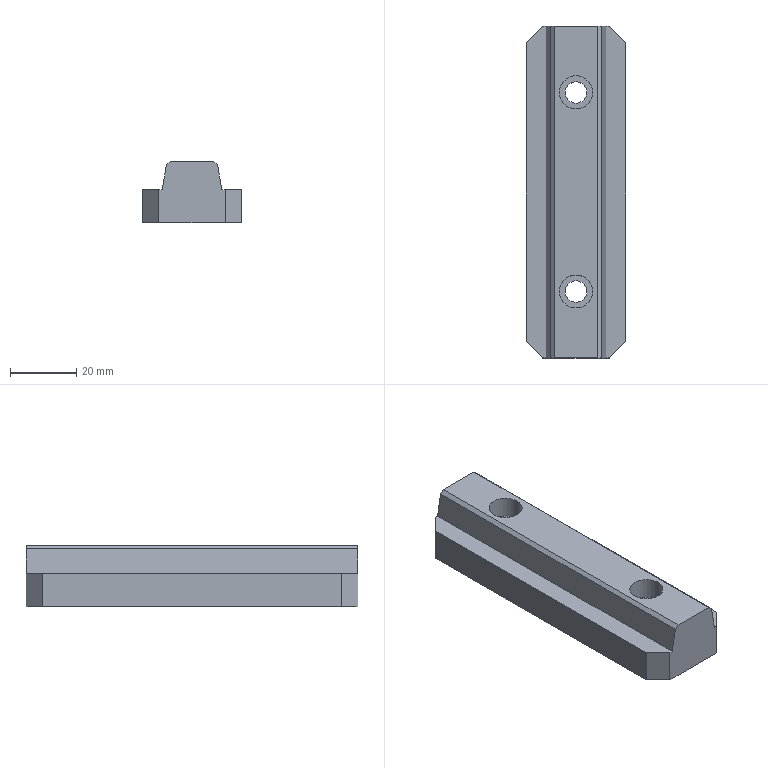Part | Creo | 1 solid | 26 faces | box 30 x 100 x 18.5 mm | volume 41610 mm3 | plane 18 | cylinder 8 | commonest cylinder face diameters 6.5 x4 10 x4
STEP:
#1=CARTESIAN_POINT('',(-253.501,30.,8.5));
#2=VERTEX_POINT('',#1);
#3=CARTESIAN_POINT('',(-240.499,30.,8.5));
#4=VERTEX_POINT('',#3);
#5=CARTESIAN_POINT('',(-253.501,30.,8.5));
#6=DIRECTION('',(1.,0.,0.));
#7=VECTOR('',#6,13.002);
#8=LINE('',#5,#7);
#9=EDGE_CURVE('',#2,#4,#8,.T.);
#10=ORIENTED_EDGE('',*,*,#9,.F.);
#11=CARTESIAN_POINT('',(-253.501,130.,8.5));
#12=VERTEX_POINT('',#11);
#13=CARTESIAN_POINT('',(-253.501,30.,8.5));
#14=DIRECTION('',(0.,1.,0.));
#15=VECTOR('',#14,100.);
#16=LINE('',#13,#15);
#17=EDGE_CURVE('',#2,#12,#16,.T.);
#18=ORIENTED_EDGE('',*,*,#17,.T.);
#19=CARTESIAN_POINT('',(-240.499,130.,8.5));
#20=VERTEX_POINT('',#19);
#21=CARTESIAN_POINT('',(-253.501,130.,8.5));
#22=DIRECTION('',(1.,0.,0.));
#23=VECTOR('',#22,13.002);
#24=LINE('',#21,#23);
#25=EDGE_CURVE('',#12,#20,#24,.T.);
#26=ORIENTED_EDGE('',*,*,#25,.T.);
#27=CARTESIAN_POINT('',(-240.499,130.,8.5));
#28=DIRECTION('',(0.,-1.,0.));
#29=VECTOR('',#28,100.);
#30=LINE('',#27,#29);
#31=EDGE_CURVE('',#20,#4,#30,.T.);
#32=ORIENTED_EDGE('',*,*,#31,.T.);
#33=EDGE_LOOP('',(#10,#18,#26,#32));
#34=FACE_OUTER_BOUND('',#33,.F.);
#35=CARTESIAN_POINT('',(-252.,50.,8.5));
#36=VERTEX_POINT('',#35);
#37=CARTESIAN_POINT('',(-242.,50.,8.5));
#38=VERTEX_POINT('',#37);
#39=CARTESIAN_POINT('',(-247.,50.,8.5));
#40=DIRECTION('',(0.,0.,-1.));
#41=DIRECTION('',(-1.,0.,0.));
#42=AXIS2_PLACEMENT_3D('',#39,#40,#41);
#43=CIRCLE('',#42,5.);
#44=EDGE_CURVE('',#36,#38,#43,.T.);
#45=ORIENTED_EDGE('',*,*,#44,.F.);
#46=CARTESIAN_POINT('',(-247.,50.,8.5));
#47=DIRECTION('',(0.,0.,-1.));
#48=DIRECTION('',(1.,0.,0.));
#49=AXIS2_PLACEMENT_3D('',#46,#47,#48);
#50=CIRCLE('',#49,5.);
#51=EDGE_CURVE('',#38,#36,#50,.T.);
#52=ORIENTED_EDGE('',*,*,#51,.F.);
#53=EDGE_LOOP('',(#45,#52));
#54=FACE_BOUND('',#53,.F.);
#55=CARTESIAN_POINT('',(-252.,110.,8.5));
#56=VERTEX_POINT('',#55);
#57=CARTESIAN_POINT('',(-242.,110.,8.5));
#58=VERTEX_POINT('',#57);
#59=CARTESIAN_POINT('',(-247.,110.,8.5));
#60=DIRECTION('',(0.,0.,-1.));
#61=DIRECTION('',(-1.,0.,0.));
#62=AXIS2_PLACEMENT_3D('',#59,#60,#61);
#63=CIRCLE('',#62,5.);
#64=EDGE_CURVE('',#56,#58,#63,.T.);
#65=ORIENTED_EDGE('',*,*,#64,.F.);
#66=CARTESIAN_POINT('',(-247.,110.,8.5));
#67=DIRECTION('',(0.,0.,-1.));
#68=DIRECTION('',(1.,0.,0.));
#69=AXIS2_PLACEMENT_3D('',#66,#67,#68);
#70=CIRCLE('',#69,5.);
#71=EDGE_CURVE('',#58,#56,#70,.T.);
#72=ORIENTED_EDGE('',*,*,#71,.F.);
#73=EDGE_LOOP('',(#65,#72));
#74=FACE_BOUND('',#73,.F.);
#75=CARTESIAN_POINT('',(-239.499,130.,8.5));
#76=DIRECTION('',(0.,0.,1.));
#77=DIRECTION('',(1.,0.,0.));
#78=AXIS2_PLACEMENT_3D('',#75,#76,#77);
#79=PLANE('',#78);
#80=ADVANCED_FACE('',(#34,#54,#74),#79,.T.);
#81=CARTESIAN_POINT('',(-242.,50.,2.));
#82=VERTEX_POINT('',#81);
#83=CARTESIAN_POINT('',(-252.,50.,2.));
#84=VERTEX_POINT('',#83);
#85=CARTESIAN_POINT('',(-247.,50.,2.));
#86=DIRECTION('',(0.,0.,1.));
#87=DIRECTION('',(1.,0.,0.));
#88=AXIS2_PLACEMENT_3D('',#85,#86,#87);
#89=CIRCLE('',#88,5.);
#90=EDGE_CURVE('',#82,#84,#89,.T.);
#91=ORIENTED_EDGE('',*,*,#90,.T.);
#92=CARTESIAN_POINT('',(-252.,50.,8.5));
#93=DIRECTION('',(0.,0.,-1.));
#94=VECTOR('',#93,6.5);
#95=LINE('',#92,#94);
#96=EDGE_CURVE('',#36,#84,#95,.T.);
#97=ORIENTED_EDGE('',*,*,#96,.F.);
#98=ORIENTED_EDGE('',*,*,#44,.T.);
#99=CARTESIAN_POINT('',(-242.,50.,8.5));
#100=DIRECTION('',(0.,0.,-1.));
#101=VECTOR('',#100,6.5);
#102=LINE('',#99,#101);
#103=EDGE_CURVE('',#38,#82,#102,.T.);
#104=ORIENTED_EDGE('',*,*,#103,.T.);
#105=EDGE_LOOP('',(#91,#97,#98,#104));
#106=FACE_OUTER_BOUND('',#105,.F.);
#107=CARTESIAN_POINT('',(-247.,50.,8.5));
#108=DIRECTION('',(0.,0.,-1.));
#109=DIRECTION('',(-1.,0.,0.));
#110=AXIS2_PLACEMENT_3D('',#107,#108,#109);
#111=CYLINDRICAL_SURFACE('',#110,5.);
#112=ADVANCED_FACE('',(#106),#111,.F.);
#113=ORIENTED_EDGE('',*,*,#90,.F.);
#114=CARTESIAN_POINT('',(-247.,50.,2.));
#115=DIRECTION('',(0.,0.,1.));
#116=DIRECTION('',(-1.,0.,0.));
#117=AXIS2_PLACEMENT_3D('',#114,#115,#116);
#118=CIRCLE('',#117,5.);
#119=EDGE_CURVE('',#84,#82,#118,.T.);
#120=ORIENTED_EDGE('',*,*,#119,.F.);
#121=EDGE_LOOP('',(#113,#120));
#122=FACE_OUTER_BOUND('',#121,.F.);
#123=CARTESIAN_POINT('',(-250.25,50.,2.));
#124=VERTEX_POINT('',#123);
#125=CARTESIAN_POINT('',(-243.75,50.,2.));
#126=VERTEX_POINT('',#125);
#127=CARTESIAN_POINT('',(-247.,50.,2.));
#128=DIRECTION('',(0.,0.,-1.));
#129=DIRECTION('',(-1.,0.,0.));
#130=AXIS2_PLACEMENT_3D('',#127,#128,#129);
#131=CIRCLE('',#130,3.25);
#132=EDGE_CURVE('',#124,#126,#131,.T.);
#133=ORIENTED_EDGE('',*,*,#132,.F.);
#134=CARTESIAN_POINT('',(-247.,50.,2.));
#135=DIRECTION('',(0.,0.,-1.));
#136=DIRECTION('',(1.,0.,0.));
#137=AXIS2_PLACEMENT_3D('',#134,#135,#136);
#138=CIRCLE('',#137,3.25);
#139=EDGE_CURVE('',#126,#124,#138,.T.);
#140=ORIENTED_EDGE('',*,*,#139,.F.);
#141=EDGE_LOOP('',(#133,#140));
#142=FACE_BOUND('',#141,.F.);
#143=CARTESIAN_POINT('',(-247.,50.,2.));
#144=DIRECTION('',(0.,0.,-1.));
#145=DIRECTION('',(-1.,0.,0.));
#146=AXIS2_PLACEMENT_3D('',#143,#144,#145);
#147=PLANE('',#146);
#148=ADVANCED_FACE('',(#122,#142),#147,.F.);
#149=ORIENTED_EDGE('',*,*,#119,.T.);
#150=ORIENTED_EDGE('',*,*,#103,.F.);
#151=ORIENTED_EDGE('',*,*,#51,.T.);
#152=ORIENTED_EDGE('',*,*,#96,.T.);
#153=EDGE_LOOP('',(#149,#150,#151,#152));
#154=FACE_OUTER_BOUND('',#153,.F.);
#155=CARTESIAN_POINT('',(-247.,50.,8.5));
#156=DIRECTION('',(0.,0.,-1.));
#157=DIRECTION('',(-1.,0.,0.));
#158=AXIS2_PLACEMENT_3D('',#155,#156,#157);
#159=CYLINDRICAL_SURFACE('',#158,5.);
#160=ADVANCED_FACE('',(#154),#159,.F.);
#161=ORIENTED_EDGE('',*,*,#132,.T.);
#162=CARTESIAN_POINT('',(-243.75,50.,-10.));
#163=VERTEX_POINT('',#162);
#164=CARTESIAN_POINT('',(-243.75,50.,2.));
#165=DIRECTION('',(0.,0.,-1.));
#166=VECTOR('',#165,12.);
#167=LINE('',#164,#166);
#168=EDGE_CURVE('',#126,#163,#167,.T.);
#169=ORIENTED_EDGE('',*,*,#168,.T.);
#170=CARTESIAN_POINT('',(-250.25,50.,-10.));
#171=VERTEX_POINT('',#170);
#172=CARTESIAN_POINT('',(-247.,50.,-10.));
#173=DIRECTION('',(0.,0.,1.));
#174=DIRECTION('',(1.,0.,0.));
#175=AXIS2_PLACEMENT_3D('',#172,#173,#174);
#176=CIRCLE('',#175,3.25);
#177=EDGE_CURVE('',#163,#171,#176,.T.);
#178=ORIENTED_EDGE('',*,*,#177,.T.);
#179=CARTESIAN_POINT('',(-250.25,50.,2.));
#180=DIRECTION('',(0.,0.,-1.));
#181=VECTOR('',#180,12.);
#182=LINE('',#179,#181);
#183=EDGE_CURVE('',#124,#171,#182,.T.);
#184=ORIENTED_EDGE('',*,*,#183,.F.);
#185=EDGE_LOOP('',(#161,#169,#178,#184));
#186=FACE_OUTER_BOUND('',#185,.F.);
#187=CARTESIAN_POINT('',(-247.,50.,8.5));
#188=DIRECTION('',(0.,0.,-1.));
#189=DIRECTION('',(-1.,0.,0.));
#190=AXIS2_PLACEMENT_3D('',#187,#188,#189);
#191=CYLINDRICAL_SURFACE('',#190,3.25);
#192=ADVANCED_FACE('',(#186),#191,.F.);
#193=ORIENTED_EDGE('',*,*,#139,.T.);
#194=ORIENTED_EDGE('',*,*,#183,.T.);
#195=CARTESIAN_POINT('',(-247.,50.,-10.));
#196=DIRECTION('',(0.,0.,1.));
#197=DIRECTION('',(-1.,0.,0.));
#198=AXIS2_PLACEMENT_3D('',#195,#196,#197);
#199=CIRCLE('',#198,3.25);
#200=EDGE_CURVE('',#171,#163,#199,.T.);
#201=ORIENTED_EDGE('',*,*,#200,.T.);
#202=ORIENTED_EDGE('',*,*,#168,.F.);
#203=EDGE_LOOP('',(#193,#194,#201,#202));
#204=FACE_OUTER_BOUND('',#203,.F.);
#205=CARTESIAN_POINT('',(-247.,50.,8.5));
#206=DIRECTION('',(0.,0.,-1.));
#207=DIRECTION('',(-1.,0.,0.));
#208=AXIS2_PLACEMENT_3D('',#205,#206,#207);
#209=CYLINDRICAL_SURFACE('',#208,3.25);
#210=ADVANCED_FACE('',(#204),#209,.F.);
#211=CARTESIAN_POINT('',(-262.,35.,-10.));
#212=VERTEX_POINT('',#211);
#213=CARTESIAN_POINT('',(-262.,125.,-10.));
#214=VERTEX_POINT('',#213);
#215=CARTESIAN_POINT('',(-262.,35.,-10.));
#216=DIRECTION('',(0.,1.,0.));
#217=VECTOR('',#216,90.);
#218=LINE('',#215,#217);
#219=EDGE_CURVE('',#212,#214,#218,.T.);
#220=ORIENTED_EDGE('',*,*,#219,.F.);
#221=CARTESIAN_POINT('',(-257.,30.,-10.));
#222=VERTEX_POINT('',#221);
#223=CARTESIAN_POINT('',(-257.,30.,-10.));
#224=DIRECTION('',(-0.7071,0.7071,0.));
#225=VECTOR('',#224,7.071);
#226=LINE('',#223,#225);
#227=EDGE_CURVE('',#222,#212,#226,.T.);
#228=ORIENTED_EDGE('',*,*,#227,.F.);
#229=CARTESIAN_POINT('',(-237.,30.,-10.));
#230=VERTEX_POINT('',#229);
#231=CARTESIAN_POINT('',(-237.,30.,-10.));
#232=DIRECTION('',(-1.,0.,0.));
#233=VECTOR('',#232,20.);
#234=LINE('',#231,#233);
#235=EDGE_CURVE('',#230,#222,#234,.T.);
#236=ORIENTED_EDGE('',*,*,#235,.F.);
#237=CARTESIAN_POINT('',(-232.,35.,-10.));
#238=VERTEX_POINT('',#237);
#239=CARTESIAN_POINT('',(-232.,35.,-10.));
#240=DIRECTION('',(-0.7071,-0.7071,0.));
#241=VECTOR('',#240,7.071);
#242=LINE('',#239,#241);
#243=EDGE_CURVE('',#238,#230,#242,.T.);
#244=ORIENTED_EDGE('',*,*,#243,.F.);
#245=CARTESIAN_POINT('',(-232.,125.,-10.));
#246=VERTEX_POINT('',#245);
#247=CARTESIAN_POINT('',(-232.,125.,-10.));
#248=DIRECTION('',(0.,-1.,0.));
#249=VECTOR('',#248,90.);
#250=LINE('',#247,#249);
#251=EDGE_CURVE('',#246,#238,#250,.T.);
#252=ORIENTED_EDGE('',*,*,#251,.F.);
#253=CARTESIAN_POINT('',(-237.,130.,-10.));
#254=VERTEX_POINT('',#253);
#255=CARTESIAN_POINT('',(-237.,130.,-10.));
#256=DIRECTION('',(0.7071,-0.7071,0.));
#257=VECTOR('',#256,7.071);
#258=LINE('',#255,#257);
#259=EDGE_CURVE('',#254,#246,#258,.T.);
#260=ORIENTED_EDGE('',*,*,#259,.F.);
#261=CARTESIAN_POINT('',(-257.,130.,-10.));
#262=VERTEX_POINT('',#261);
#263=CARTESIAN_POINT('',(-257.,130.,-10.));
#264=DIRECTION('',(1.,0.,0.));
#265=VECTOR('',#264,20.);
#266=LINE('',#263,#265);
#267=EDGE_CURVE('',#262,#254,#266,.T.);
#268=ORIENTED_EDGE('',*,*,#267,.F.);
#269=CARTESIAN_POINT('',(-262.,125.,-10.));
#270=DIRECTION('',(0.7071,0.7071,0.));
#271=VECTOR('',#270,7.071);
#272=LINE('',#269,#271);
#273=EDGE_CURVE('',#214,#262,#272,.T.);
#274=ORIENTED_EDGE('',*,*,#273,.F.);
#275=EDGE_LOOP('',(#220,#228,#236,#244,#252,#260,#268,#274));
#276=FACE_OUTER_BOUND('',#275,.F.);
#277=CARTESIAN_POINT('',(-243.75,110.,-10.));
#278=VERTEX_POINT('',#277);
#279=CARTESIAN_POINT('',(-250.25,110.,-10.));
#280=VERTEX_POINT('',#279);
#281=CARTESIAN_POINT('',(-247.,110.,-10.));
#282=DIRECTION('',(0.,0.,1.));
#283=DIRECTION('',(1.,0.,0.));
#284=AXIS2_PLACEMENT_3D('',#281,#282,#283);
#285=CIRCLE('',#284,3.25);
#286=EDGE_CURVE('',#278,#280,#285,.T.);
#287=ORIENTED_EDGE('',*,*,#286,.F.);
#288=CARTESIAN_POINT('',(-247.,110.,-10.));
#289=DIRECTION('',(0.,0.,1.));
#290=DIRECTION('',(-1.,0.,0.));
#291=AXIS2_PLACEMENT_3D('',#288,#289,#290);
#292=CIRCLE('',#291,3.25);
#293=EDGE_CURVE('',#280,#278,#292,.T.);
#294=ORIENTED_EDGE('',*,*,#293,.F.);
#295=EDGE_LOOP('',(#287,#294));
#296=FACE_BOUND('',#295,.F.);
#297=ORIENTED_EDGE('',*,*,#177,.F.);
#298=ORIENTED_EDGE('',*,*,#200,.F.);
#299=EDGE_LOOP('',(#297,#298));
#300=FACE_BOUND('',#299,.F.);
#301=CARTESIAN_POINT('',(-247.,80.,-10.));
#302=DIRECTION('',(0.,0.,-1.));
#303=DIRECTION('',(-1.,0.,0.));
#304=AXIS2_PLACEMENT_3D('',#301,#302,#303);
#305=PLANE('',#304);
#306=ADVANCED_FACE('',(#276,#296,#300),#305,.T.);
#307=CARTESIAN_POINT('',(-262.,125.,0.));
#308=VERTEX_POINT('',#307);
#309=CARTESIAN_POINT('',(-262.,35.,0.));
#310=VERTEX_POINT('',#309);
#311=CARTESIAN_POINT('',(-262.,125.,0.));
#312=DIRECTION('',(0.,-1.,0.));
#313=VECTOR('',#312,90.);
#314=LINE('',#311,#313);
#315=EDGE_CURVE('',#308,#310,#314,.T.);
#316=ORIENTED_EDGE('',*,*,#315,.T.);
#317=CARTESIAN_POINT('',(-262.,35.,0.));
#318=DIRECTION('',(0.,0.,-1.));
#319=VECTOR('',#318,10.);
#320=LINE('',#317,#319);
#321=EDGE_CURVE('',#310,#212,#320,.T.);
#322=ORIENTED_EDGE('',*,*,#321,.T.);
#323=ORIENTED_EDGE('',*,*,#219,.T.);
#324=CARTESIAN_POINT('',(-262.,125.,-10.));
#325=DIRECTION('',(0.,0.,1.));
#326=VECTOR('',#325,10.);
#327=LINE('',#324,#326);
#328=EDGE_CURVE('',#214,#308,#327,.T.);
#329=ORIENTED_EDGE('',*,*,#328,.T.);
#330=EDGE_LOOP('',(#316,#322,#323,#329));
#331=FACE_OUTER_BOUND('',#330,.F.);
#332=CARTESIAN_POINT('',(-262.,80.,-10.));
#333=DIRECTION('',(-1.,0.,0.));
#334=DIRECTION('',(0.,0.,1.));
#335=AXIS2_PLACEMENT_3D('',#332,#333,#334);
#336=PLANE('',#335);
#337=ADVANCED_FACE('',(#331),#336,.T.);
#338=CARTESIAN_POINT('',(-256.,30.,0.));
#339=VERTEX_POINT('',#338);
#340=CARTESIAN_POINT('',(-256.,130.,0.));
#341=VERTEX_POINT('',#340);
#342=CARTESIAN_POINT('',(-256.,30.,0.));
#343=DIRECTION('',(0.,1.,0.));
#344=VECTOR('',#343,100.);
#345=LINE('',#342,#344);
#346=EDGE_CURVE('',#339,#341,#345,.T.);
#347=ORIENTED_EDGE('',*,*,#346,.F.);
#348=CARTESIAN_POINT('',(-257.,30.,0.));
#349=VERTEX_POINT('',#348);
#350=CARTESIAN_POINT('',(-257.,30.,0.));
#351=DIRECTION('',(1.,0.,0.));
#352=VECTOR('',#351,1.);
#353=LINE('',#350,#352);
#354=EDGE_CURVE('',#349,#339,#353,.T.);
#355=ORIENTED_EDGE('',*,*,#354,.F.);
#356=CARTESIAN_POINT('',(-262.,35.,0.));
#357=DIRECTION('',(0.7071,-0.7071,0.));
#358=VECTOR('',#357,7.071);
#359=LINE('',#356,#358);
#360=EDGE_CURVE('',#310,#349,#359,.T.);
#361=ORIENTED_EDGE('',*,*,#360,.F.);
#362=ORIENTED_EDGE('',*,*,#315,.F.);
#363=CARTESIAN_POINT('',(-257.,130.,0.));
#364=VERTEX_POINT('',#363);
#365=CARTESIAN_POINT('',(-257.,130.,0.));
#366=DIRECTION('',(-0.7071,-0.7071,0.));
#367=VECTOR('',#366,7.071);
#368=LINE('',#365,#367);
#369=EDGE_CURVE('',#364,#308,#368,.T.);
#370=ORIENTED_EDGE('',*,*,#369,.F.);
#371=CARTESIAN_POINT('',(-256.,130.,0.));
#372=DIRECTION('',(-1.,0.,0.));
#373=VECTOR('',#372,1.);
#374=LINE('',#371,#373);
#375=EDGE_CURVE('',#341,#364,#374,.T.);
#376=ORIENTED_EDGE('',*,*,#375,.F.);
#377=EDGE_LOOP('',(#347,#355,#361,#362,#370,#376));
#378=FACE_OUTER_BOUND('',#377,.F.);
#379=CARTESIAN_POINT('',(-247.,80.,0.));
#380=DIRECTION('',(0.,0.,1.));
#381=DIRECTION('',(1.,0.,0.));
#382=AXIS2_PLACEMENT_3D('',#379,#380,#381);
#383=PLANE('',#382);
#384=ADVANCED_FACE('',(#378),#383,.T.);
#385=CARTESIAN_POINT('',(-254.675,30.,7.515));
#386=VERTEX_POINT('',#385);
#387=CARTESIAN_POINT('',(-254.675,30.,7.515));
#388=DIRECTION('',(-0.1736,0.,-0.9848));
#389=VECTOR('',#388,7.631);
#390=LINE('',#387,#389);
#391=EDGE_CURVE('',#386,#339,#390,.T.);
#392=ORIENTED_EDGE('',*,*,#391,.T.);
#393=ORIENTED_EDGE('',*,*,#346,.T.);
#394=CARTESIAN_POINT('',(-254.675,130.,7.515));
#395=VERTEX_POINT('',#394);
#396=CARTESIAN_POINT('',(-256.,130.,0.));
#397=DIRECTION('',(0.1736,0.,0.9848));
#398=VECTOR('',#397,7.631);
#399=LINE('',#396,#398);
#400=EDGE_CURVE('',#341,#395,#399,.T.);
#401=ORIENTED_EDGE('',*,*,#400,.T.);
#402=CARTESIAN_POINT('',(-254.675,130.,7.515));
#403=DIRECTION('',(0.,-1.,0.));
#404=VECTOR('',#403,100.);
#405=LINE('',#402,#404);
#406=EDGE_CURVE('',#395,#386,#405,.T.);
#407=ORIENTED_EDGE('',*,*,#406,.T.);
#408=EDGE_LOOP('',(#392,#393,#401,#407));
#409=FACE_OUTER_BOUND('',#408,.F.);
#410=CARTESIAN_POINT('',(-254.501,130.,8.5));
#411=DIRECTION('',(-0.9848,0.,0.1736));
#412=DIRECTION('',(0.1736,0.,0.9848));
#413=AXIS2_PLACEMENT_3D('',#410,#411,#412);
#414=PLANE('',#413);
#415=ADVANCED_FACE('',(#409),#414,.T.);
#416=CARTESIAN_POINT('',(-238.,30.,0.));
#417=VERTEX_POINT('',#416);
#418=CARTESIAN_POINT('',(-239.325,30.,7.515));
#419=VERTEX_POINT('',#418);
#420=CARTESIAN_POINT('',(-238.,30.,0.));
#421=DIRECTION('',(-0.1736,0.,0.9848));
#422=VECTOR('',#421,7.631);
#423=LINE('',#420,#422);
#424=EDGE_CURVE('',#417,#419,#423,.T.);
#425=ORIENTED_EDGE('',*,*,#424,.F.);
#426=CARTESIAN_POINT('',(-237.,30.,0.));
#427=VERTEX_POINT('',#426);
#428=CARTESIAN_POINT('',(-238.,30.,0.));
#429=DIRECTION('',(1.,0.,0.));
#430=VECTOR('',#429,1.);
#431=LINE('',#428,#430);
#432=EDGE_CURVE('',#417,#427,#431,.T.);
#433=ORIENTED_EDGE('',*,*,#432,.T.);
#434=CARTESIAN_POINT('',(-237.,30.,0.));
#435=DIRECTION('',(0.,0.,-1.));
#436=VECTOR('',#435,10.);
#437=LINE('',#434,#436);
#438=EDGE_CURVE('',#427,#230,#437,.T.);
#439=ORIENTED_EDGE('',*,*,#438,.T.);
#440=ORIENTED_EDGE('',*,*,#235,.T.);
#441=CARTESIAN_POINT('',(-257.,30.,-10.));
#442=DIRECTION('',(0.,0.,1.));
#443=VECTOR('',#442,10.);
#444=LINE('',#441,#443);
#445=EDGE_CURVE('',#222,#349,#444,.T.);
#446=ORIENTED_EDGE('',*,*,#445,.T.);
#447=ORIENTED_EDGE('',*,*,#354,.T.);
#448=ORIENTED_EDGE('',*,*,#391,.F.);
#449=CARTESIAN_POINT('',(-253.501,30.,8.5));
#450=DIRECTION('',(-0.766,0.,-0.6428));
#451=VECTOR('',#450,1.532);
#452=LINE('',#449,#451);
#453=EDGE_CURVE('',#2,#386,#452,.T.);
#454=ORIENTED_EDGE('',*,*,#453,.F.);
#455=ORIENTED_EDGE('',*,*,#9,.T.);
#456=CARTESIAN_POINT('',(-239.325,30.,7.515));
#457=DIRECTION('',(-0.766,0.,0.6428));
#458=VECTOR('',#457,1.532);
#459=LINE('',#456,#458);
#460=EDGE_CURVE('',#419,#4,#459,.T.);
#461=ORIENTED_EDGE('',*,*,#460,.F.);
#462=EDGE_LOOP('',(#425,#433,#439,#440,#446,#447,#448,#454,#455,#461));
#463=FACE_OUTER_BOUND('',#462,.F.);
#464=CARTESIAN_POINT('',(-247.,30.,-10.));
#465=DIRECTION('',(0.,-1.,0.));
#466=DIRECTION('',(0.,0.,-1.));
#467=AXIS2_PLACEMENT_3D('',#464,#465,#466);
#468=PLANE('',#467);
#469=ADVANCED_FACE('',(#463),#468,.T.);
#470=CARTESIAN_POINT('',(-239.325,130.,7.515));
#471=VERTEX_POINT('',#470);
#472=CARTESIAN_POINT('',(-238.,130.,0.));
#473=VERTEX_POINT('',#472);
#474=CARTESIAN_POINT('',(-239.325,130.,7.515));
#475=DIRECTION('',(0.1736,0.,-0.9848));
#476=VECTOR('',#475,7.631);
#477=LINE('',#474,#476);
#478=EDGE_CURVE('',#471,#473,#477,.T.);
#479=ORIENTED_EDGE('',*,*,#478,.T.);
#480=CARTESIAN_POINT('',(-238.,30.,0.));
#481=DIRECTION('',(0.,1.,0.));
#482=VECTOR('',#481,100.);
#483=LINE('',#480,#482);
#484=EDGE_CURVE('',#417,#473,#483,.T.);
#485=ORIENTED_EDGE('',*,*,#484,.F.);
#486=ORIENTED_EDGE('',*,*,#424,.T.);
#487=CARTESIAN_POINT('',(-239.325,30.,7.515));
#488=DIRECTION('',(0.,1.,0.));
#489=VECTOR('',#488,100.);
#490=LINE('',#487,#489);
#491=EDGE_CURVE('',#419,#471,#490,.T.);
#492=ORIENTED_EDGE('',*,*,#491,.T.);
#493=EDGE_LOOP('',(#479,#485,#486,#492));
#494=FACE_OUTER_BOUND('',#493,.F.);
#495=CARTESIAN_POINT('',(-238.,130.,0.));
#496=DIRECTION('',(0.9848,0.,0.1736));
#497=DIRECTION('',(0.1736,0.,-0.9848));
#498=AXIS2_PLACEMENT_3D('',#495,#496,#497);
#499=PLANE('',#498);
#500=ADVANCED_FACE('',(#494),#499,.T.);
#501=ORIENTED_EDGE('',*,*,#25,.F.);
#502=CARTESIAN_POINT('',(-254.675,130.,7.515));
#503=DIRECTION('',(0.766,0.,0.6428));
#504=VECTOR('',#503,1.532);
#505=LINE('',#502,#504);
#506=EDGE_CURVE('',#395,#12,#505,.T.);
#507=ORIENTED_EDGE('',*,*,#506,.F.);
#508=ORIENTED_EDGE('',*,*,#400,.F.);
#509=ORIENTED_EDGE('',*,*,#375,.T.);
#510=CARTESIAN_POINT('',(-257.,130.,0.));
#511=DIRECTION('',(0.,0.,-1.));
#512=VECTOR('',#511,10.);
#513=LINE('',#510,#512);
#514=EDGE_CURVE('',#364,#262,#513,.T.);
#515=ORIENTED_EDGE('',*,*,#514,.T.);
#516=ORIENTED_EDGE('',*,*,#267,.T.);
#517=CARTESIAN_POINT('',(-237.,130.,0.));
#518=VERTEX_POINT('',#517);
#519=CARTESIAN_POINT('',(-237.,130.,-10.));
#520=DIRECTION('',(0.,0.,1.));
#521=VECTOR('',#520,10.);
#522=LINE('',#519,#521);
#523=EDGE_CURVE('',#254,#518,#522,.T.);
#524=ORIENTED_EDGE('',*,*,#523,.T.);
#525=CARTESIAN_POINT('',(-237.,130.,0.));
#526=DIRECTION('',(-1.,0.,0.));
#527=VECTOR('',#526,1.);
#528=LINE('',#525,#527);
#529=EDGE_CURVE('',#518,#473,#528,.T.);
#530=ORIENTED_EDGE('',*,*,#529,.T.);
#531=ORIENTED_EDGE('',*,*,#478,.F.);
#532=CARTESIAN_POINT('',(-240.499,130.,8.5));
#533=DIRECTION('',(0.766,0.,-0.6428));
#534=VECTOR('',#533,1.532);
#535=LINE('',#532,#534);
#536=EDGE_CURVE('',#20,#471,#535,.T.);
#537=ORIENTED_EDGE('',*,*,#536,.F.);
#538=EDGE_LOOP('',(#501,#507,#508,#509,#515,#516,#524,#530,#531,#537));
#539=FACE_OUTER_BOUND('',#538,.F.);
#540=CARTESIAN_POINT('',(-247.,130.,-10.));
#541=DIRECTION('',(0.,1.,0.));
#542=DIRECTION('',(0.,0.,1.));
#543=AXIS2_PLACEMENT_3D('',#540,#541,#542);
#544=PLANE('',#543);
#545=ADVANCED_FACE('',(#539),#544,.T.);
#546=ORIENTED_EDGE('',*,*,#506,.T.);
#547=ORIENTED_EDGE('',*,*,#17,.F.);
#548=ORIENTED_EDGE('',*,*,#453,.T.);
#549=ORIENTED_EDGE('',*,*,#406,.F.);
#550=EDGE_LOOP('',(#546,#547,#548,#549));
#551=FACE_OUTER_BOUND('',#550,.F.);
#552=CARTESIAN_POINT('',(-253.501,130.,8.5));
#553=DIRECTION('',(0.6428,0.,-0.766));
#554=DIRECTION('',(-0.766,0.,-0.6428));
#555=AXIS2_PLACEMENT_3D('',#552,#553,#554);
#556=PLANE('',#555);
#557=ADVANCED_FACE('',(#551),#556,.F.);
#558=ORIENTED_EDGE('',*,*,#273,.T.);
#559=ORIENTED_EDGE('',*,*,#514,.F.);
#560=ORIENTED_EDGE('',*,*,#369,.T.);
#561=ORIENTED_EDGE('',*,*,#328,.F.);
#562=EDGE_LOOP('',(#558,#559,#560,#561));
#563=FACE_OUTER_BOUND('',#562,.F.);
#564=CARTESIAN_POINT('',(-257.,130.,-10.));
#565=DIRECTION('',(0.7071,-0.7071,0.));
#566=DIRECTION('',(0.7071,0.7071,0.));
#567=AXIS2_PLACEMENT_3D('',#564,#565,#566);
#568=PLANE('',#567);
#569=ADVANCED_FACE('',(#563),#568,.F.);
#570=ORIENTED_EDGE('',*,*,#259,.T.);
#571=CARTESIAN_POINT('',(-232.,125.,0.));
#572=VERTEX_POINT('',#571);
#573=CARTESIAN_POINT('',(-232.,125.,0.));
#574=DIRECTION('',(0.,0.,-1.));
#575=VECTOR('',#574,10.);
#576=LINE('',#573,#575);
#577=EDGE_CURVE('',#572,#246,#576,.T.);
#578=ORIENTED_EDGE('',*,*,#577,.F.);
#579=CARTESIAN_POINT('',(-232.,125.,0.));
#580=DIRECTION('',(-0.7071,0.7071,0.));
#581=VECTOR('',#580,7.071);
#582=LINE('',#579,#581);
#583=EDGE_CURVE('',#572,#518,#582,.T.);
#584=ORIENTED_EDGE('',*,*,#583,.T.);
#585=ORIENTED_EDGE('',*,*,#523,.F.);
#586=EDGE_LOOP('',(#570,#578,#584,#585));
#587=FACE_OUTER_BOUND('',#586,.F.);
#588=CARTESIAN_POINT('',(-232.,125.,-10.));
#589=DIRECTION('',(-0.7071,-0.7071,0.));
#590=DIRECTION('',(0.7071,-0.7071,0.));
#591=AXIS2_PLACEMENT_3D('',#588,#589,#590);
#592=PLANE('',#591);
#593=ADVANCED_FACE('',(#587),#592,.F.);
#594=ORIENTED_EDGE('',*,*,#251,.T.);
#595=CARTESIAN_POINT('',(-232.,35.,0.));
#596=VERTEX_POINT('',#595);
#597=CARTESIAN_POINT('',(-232.,35.,-10.));
#598=DIRECTION('',(0.,0.,1.));
#599=VECTOR('',#598,10.);
#600=LINE('',#597,#599);
#601=EDGE_CURVE('',#238,#596,#600,.T.);
#602=ORIENTED_EDGE('',*,*,#601,.T.);
#603=CARTESIAN_POINT('',(-232.,35.,0.));
#604=DIRECTION('',(0.,1.,0.));
#605=VECTOR('',#604,90.);
#606=LINE('',#603,#605);
#607=EDGE_CURVE('',#596,#572,#606,.T.);
#608=ORIENTED_EDGE('',*,*,#607,.T.);
#609=ORIENTED_EDGE('',*,*,#577,.T.);
#610=EDGE_LOOP('',(#594,#602,#608,#609));
#611=FACE_OUTER_BOUND('',#610,.F.);
#612=CARTESIAN_POINT('',(-232.,80.,-10.));
#613=DIRECTION('',(1.,0.,0.));
#614=DIRECTION('',(0.,0.,-1.));
#615=AXIS2_PLACEMENT_3D('',#612,#613,#614);
#616=PLANE('',#615);
#617=ADVANCED_FACE('',(#611),#616,.T.);
#618=ORIENTED_EDGE('',*,*,#243,.T.);
#619=ORIENTED_EDGE('',*,*,#438,.F.);
#620=CARTESIAN_POINT('',(-237.,30.,0.));
#621=DIRECTION('',(0.7071,0.7071,0.));
#622=VECTOR('',#621,7.071);
#623=LINE('',#620,#622);
#624=EDGE_CURVE('',#427,#596,#623,.T.);
#625=ORIENTED_EDGE('',*,*,#624,.T.);
#626=ORIENTED_EDGE('',*,*,#601,.F.);
#627=EDGE_LOOP('',(#618,#619,#625,#626));
#628=FACE_OUTER_BOUND('',#627,.F.);
#629=CARTESIAN_POINT('',(-237.,30.,-10.));
#630=DIRECTION('',(-0.7071,0.7071,0.));
#631=DIRECTION('',(-0.7071,-0.7071,0.));
#632=AXIS2_PLACEMENT_3D('',#629,#630,#631);
#633=PLANE('',#632);
#634=ADVANCED_FACE('',(#628),#633,.F.);
#635=ORIENTED_EDGE('',*,*,#529,.F.);
#636=ORIENTED_EDGE('',*,*,#583,.F.);
#637=ORIENTED_EDGE('',*,*,#607,.F.);
#638=ORIENTED_EDGE('',*,*,#624,.F.);
#639=ORIENTED_EDGE('',*,*,#432,.F.);
#640=ORIENTED_EDGE('',*,*,#484,.T.);
#641=EDGE_LOOP('',(#635,#636,#637,#638,#639,#640));
#642=FACE_OUTER_BOUND('',#641,.F.);
#643=CARTESIAN_POINT('',(-247.,80.,0.));
#644=DIRECTION('',(0.,0.,1.));
#645=DIRECTION('',(1.,0.,0.));
#646=AXIS2_PLACEMENT_3D('',#643,#644,#645);
#647=PLANE('',#646);
#648=ADVANCED_FACE('',(#642),#647,.T.);
#649=ORIENTED_EDGE('',*,*,#536,.T.);
#650=ORIENTED_EDGE('',*,*,#491,.F.);
#651=ORIENTED_EDGE('',*,*,#460,.T.);
#652=ORIENTED_EDGE('',*,*,#31,.F.);
#653=EDGE_LOOP('',(#649,#650,#651,#652));
#654=FACE_OUTER_BOUND('',#653,.F.);
#655=CARTESIAN_POINT('',(-239.325,130.,7.515));
#656=DIRECTION('',(-0.6428,0.,-0.766));
#657=DIRECTION('',(-0.766,0.,0.6428));
#658=AXIS2_PLACEMENT_3D('',#655,#656,#657);
#659=PLANE('',#658);
#660=ADVANCED_FACE('',(#654),#659,.F.);
#661=ORIENTED_EDGE('',*,*,#227,.T.);
#662=ORIENTED_EDGE('',*,*,#321,.F.);
#663=ORIENTED_EDGE('',*,*,#360,.T.);
#664=ORIENTED_EDGE('',*,*,#445,.F.);
#665=EDGE_LOOP('',(#661,#662,#663,#664));
#666=FACE_OUTER_BOUND('',#665,.F.);
#667=CARTESIAN_POINT('',(-262.,35.,-10.));
#668=DIRECTION('',(0.7071,0.7071,0.));
#669=DIRECTION('',(-0.7071,0.7071,0.));
#670=AXIS2_PLACEMENT_3D('',#667,#668,#669);
#671=PLANE('',#670);
#672=ADVANCED_FACE('',(#666),#671,.F.);
#673=CARTESIAN_POINT('',(-250.25,110.,2.));
#674=VERTEX_POINT('',#673);
#675=CARTESIAN_POINT('',(-243.75,110.,2.));
#676=VERTEX_POINT('',#675);
#677=CARTESIAN_POINT('',(-247.,110.,2.));
#678=DIRECTION('',(0.,0.,-1.));
#679=DIRECTION('',(-1.,0.,0.));
#680=AXIS2_PLACEMENT_3D('',#677,#678,#679);
#681=CIRCLE('',#680,3.25);
#682=EDGE_CURVE('',#674,#676,#681,.T.);
#683=ORIENTED_EDGE('',*,*,#682,.T.);
#684=CARTESIAN_POINT('',(-243.75,110.,2.));
#685=DIRECTION('',(0.,0.,-1.));
#686=VECTOR('',#685,12.);
#687=LINE('',#684,#686);
#688=EDGE_CURVE('',#676,#278,#687,.T.);
#689=ORIENTED_EDGE('',*,*,#688,.T.);
#690=ORIENTED_EDGE('',*,*,#286,.T.);
#691=CARTESIAN_POINT('',(-250.25,110.,2.));
#692=DIRECTION('',(0.,0.,-1.));
#693=VECTOR('',#692,12.);
#694=LINE('',#691,#693);
#695=EDGE_CURVE('',#674,#280,#694,.T.);
#696=ORIENTED_EDGE('',*,*,#695,.F.);
#697=EDGE_LOOP('',(#683,#689,#690,#696));
#698=FACE_OUTER_BOUND('',#697,.F.);
#699=CARTESIAN_POINT('',(-247.,110.,8.5));
#700=DIRECTION('',(0.,0.,-1.));
#701=DIRECTION('',(-1.,0.,0.));
#702=AXIS2_PLACEMENT_3D('',#699,#700,#701);
#703=CYLINDRICAL_SURFACE('',#702,3.25);
#704=ADVANCED_FACE('',(#698),#703,.F.);
#705=CARTESIAN_POINT('',(-242.,110.,2.));
#706=VERTEX_POINT('',#705);
#707=CARTESIAN_POINT('',(-252.,110.,2.));
#708=VERTEX_POINT('',#707);
#709=CARTESIAN_POINT('',(-247.,110.,2.));
#710=DIRECTION('',(0.,0.,1.));
#711=DIRECTION('',(1.,0.,0.));
#712=AXIS2_PLACEMENT_3D('',#709,#710,#711);
#713=CIRCLE('',#712,5.);
#714=EDGE_CURVE('',#706,#708,#713,.T.);
#715=ORIENTED_EDGE('',*,*,#714,.F.);
#716=CARTESIAN_POINT('',(-247.,110.,2.));
#717=DIRECTION('',(0.,0.,1.));
#718=DIRECTION('',(-1.,0.,0.));
#719=AXIS2_PLACEMENT_3D('',#716,#717,#718);
#720=CIRCLE('',#719,5.);
#721=EDGE_CURVE('',#708,#706,#720,.T.);
#722=ORIENTED_EDGE('',*,*,#721,.F.);
#723=EDGE_LOOP('',(#715,#722));
#724=FACE_OUTER_BOUND('',#723,.F.);
#725=ORIENTED_EDGE('',*,*,#682,.F.);
#726=CARTESIAN_POINT('',(-247.,110.,2.));
#727=DIRECTION('',(0.,0.,-1.));
#728=DIRECTION('',(1.,0.,0.));
#729=AXIS2_PLACEMENT_3D('',#726,#727,#728);
#730=CIRCLE('',#729,3.25);
#731=EDGE_CURVE('',#676,#674,#730,.T.);
#732=ORIENTED_EDGE('',*,*,#731,.F.);
#733=EDGE_LOOP('',(#725,#732));
#734=FACE_BOUND('',#733,.F.);
#735=CARTESIAN_POINT('',(-247.,110.,2.));
#736=DIRECTION('',(0.,0.,-1.));
#737=DIRECTION('',(-1.,0.,0.));
#738=AXIS2_PLACEMENT_3D('',#735,#736,#737);
#739=PLANE('',#738);
#740=ADVANCED_FACE('',(#724,#734),#739,.F.);
#741=ORIENTED_EDGE('',*,*,#714,.T.);
#742=CARTESIAN_POINT('',(-252.,110.,8.5));
#743=DIRECTION('',(0.,0.,-1.));
#744=VECTOR('',#743,6.5);
#745=LINE('',#742,#744);
#746=EDGE_CURVE('',#56,#708,#745,.T.);
#747=ORIENTED_EDGE('',*,*,#746,.F.);
#748=ORIENTED_EDGE('',*,*,#64,.T.);
#749=CARTESIAN_POINT('',(-242.,110.,8.5));
#750=DIRECTION('',(0.,0.,-1.));
#751=VECTOR('',#750,6.5);
#752=LINE('',#749,#751);
#753=EDGE_CURVE('',#58,#706,#752,.T.);
#754=ORIENTED_EDGE('',*,*,#753,.T.);
#755=EDGE_LOOP('',(#741,#747,#748,#754));
#756=FACE_OUTER_BOUND('',#755,.F.);
#757=CARTESIAN_POINT('',(-247.,110.,8.5));
#758=DIRECTION('',(0.,0.,-1.));
#759=DIRECTION('',(-1.,0.,0.));
#760=AXIS2_PLACEMENT_3D('',#757,#758,#759);
#761=CYLINDRICAL_SURFACE('',#760,5.);
#762=ADVANCED_FACE('',(#756),#761,.F.);
#763=ORIENTED_EDGE('',*,*,#721,.T.);
#764=ORIENTED_EDGE('',*,*,#753,.F.);
#765=ORIENTED_EDGE('',*,*,#71,.T.);
#766=ORIENTED_EDGE('',*,*,#746,.T.);
#767=EDGE_LOOP('',(#763,#764,#765,#766));
#768=FACE_OUTER_BOUND('',#767,.F.);
#769=CARTESIAN_POINT('',(-247.,110.,8.5));
#770=DIRECTION('',(0.,0.,-1.));
#771=DIRECTION('',(-1.,0.,0.));
#772=AXIS2_PLACEMENT_3D('',#769,#770,#771);
#773=CYLINDRICAL_SURFACE('',#772,5.);
#774=ADVANCED_FACE('',(#768),#773,.F.);
#775=ORIENTED_EDGE('',*,*,#731,.T.);
#776=ORIENTED_EDGE('',*,*,#695,.T.);
#777=ORIENTED_EDGE('',*,*,#293,.T.);
#778=ORIENTED_EDGE('',*,*,#688,.F.);
#779=EDGE_LOOP('',(#775,#776,#777,#778));
#780=FACE_OUTER_BOUND('',#779,.F.);
#781=CARTESIAN_POINT('',(-247.,110.,8.5));
#782=DIRECTION('',(0.,0.,-1.));
#783=DIRECTION('',(-1.,0.,0.));
#784=AXIS2_PLACEMENT_3D('',#781,#782,#783);
#785=CYLINDRICAL_SURFACE('',#784,3.25);
#786=ADVANCED_FACE('',(#780),#785,.F.);
#787=CLOSED_SHELL('',(#80,#112,#148,#160,#192,#210,#306,#337,#384,#415,#469,#500,#545,#557,#569,#593,#617,#634,#648,#660,#672,#704,#740,#762,#774,#786));
#788=MANIFOLD_SOLID_BREP('',#787);
#789=(LENGTH_UNIT()NAMED_UNIT(*)SI_UNIT(.MILLI.,.METRE.));
#790=UNCERTAINTY_MEASURE_WITH_UNIT(LENGTH_MEASURE(0.0106),#789,'','');
#791=(NAMED_UNIT(*)PLANE_ANGLE_UNIT()SI_UNIT($,.RADIAN.));
#792=PLANE_ANGLE_MEASURE_WITH_UNIT(PLANE_ANGLE_MEASURE(0.01745),#791);
#793=(CONVERSION_BASED_UNIT('DEGREE',#792)NAMED_UNIT(*)PLANE_ANGLE_UNIT());
#794=(NAMED_UNIT(*)SI_UNIT($,.STERADIAN.)SOLID_ANGLE_UNIT());
#795=(GEOMETRIC_REPRESENTATION_CONTEXT(3)GLOBAL_UNCERTAINTY_ASSIGNED_CONTEXT((#790))GLOBAL_UNIT_ASSIGNED_CONTEXT((#789,#793,#794))REPRESENTATION_CONTEXT('',''));
#796=ADVANCED_BREP_SHAPE_REPRESENTATION('',(#788),#795);